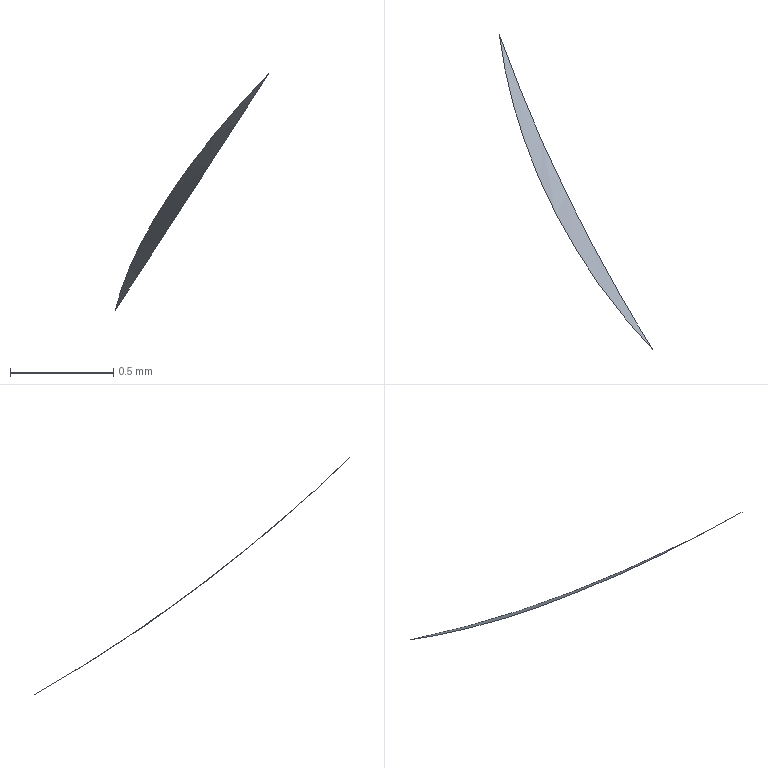Part | NX | features solid 2 | 1 solid | 2 faces | box 0.7466 x 1.533 x 1.152 mm | volume 0.001023 mm3 | cylinder 1 | spline 1 | commonest cylinder face diameters 15 x1
STEP:
#1=CARTESIAN_POINT('',(584.823,137.362,-33.981));
#2=VERTEX_POINT('',#1);
#3=CARTESIAN_POINT('',(584.077,138.895,-35.133));
#4=VERTEX_POINT('',#3);
#5=CARTESIAN_POINT('',(584.077,138.895,-35.133));
#6=CARTESIAN_POINT('',(584.194,138.576,-34.952));
#7=CARTESIAN_POINT('',(584.395,138.111,-34.642));
#8=CARTESIAN_POINT('',(584.674,137.599,-34.212));
#9=CARTESIAN_POINT('',(584.823,137.362,-33.981));
#10=B_SPLINE_CURVE_WITH_KNOTS('',3,(#5,#6,#7,#8,#9),.UNSPECIFIED.,.F.,.F.,(4,1,4),(0.4833,0.6175,0.7518),.UNSPECIFIED.);
#11=EDGE_CURVE('',#2,#4,#10,.F.);
#12=ORIENTED_EDGE('',*,*,#11,.F.);
#13=CARTESIAN_POINT('',(584.822,137.361,-33.981));
#14=CARTESIAN_POINT('',(584.437,137.772,-34.381));
#15=CARTESIAN_POINT('',(584.156,138.297,-34.794));
#16=CARTESIAN_POINT('',(584.077,138.895,-35.133));
#17=B_SPLINE_CURVE_WITH_KNOTS('',3,(#13,#14,#15,#16),.UNSPECIFIED.,.F.,.F.,(4,4),(-0.0001292,0.001944),.UNSPECIFIED.);
#18=EDGE_CURVE('',#4,#2,#17,.F.);
#19=ORIENTED_EDGE('',*,*,#18,.F.);
#20=EDGE_LOOP('',(#12,#19));
#21=FACE_BOUND('',#20,.T.);
#22=CARTESIAN_POINT('',(699.976,142.581,-28.61));
#23=DIRECTION('',(1.,-0.00013,0.000000201));
#24=DIRECTION('',(0.0001298,0.9979,0.0641));
#25=AXIS2_PLACEMENT_3D('',#22,#23,#24);
#26=CYLINDRICAL_SURFACE('',#25,7.5);
#27=ADVANCED_FACE('',(#21),#26,.T.);
#28=ORIENTED_EDGE('',*,*,#18,.T.);
#29=ORIENTED_EDGE('',*,*,#11,.T.);
#30=EDGE_LOOP('',(#28,#29));
#31=FACE_BOUND('',#30,.T.);
#32=CARTESIAN_POINT('',(584.828,137.353,-33.973));
#33=CARTESIAN_POINT('',(584.766,137.347,-33.967));
#34=CARTESIAN_POINT('',(584.704,137.341,-33.962));
#35=CARTESIAN_POINT('',(584.826,137.356,-33.976));
#36=CARTESIAN_POINT('',(584.764,137.35,-33.97));
#37=CARTESIAN_POINT('',(584.702,137.344,-33.964));
#38=CARTESIAN_POINT('',(584.824,137.359,-33.978));
#39=CARTESIAN_POINT('',(584.762,137.353,-33.973));
#40=CARTESIAN_POINT('',(584.7,137.346,-33.967));
#41=CARTESIAN_POINT('',(584.534,137.818,-34.427));
#42=CARTESIAN_POINT('',(584.472,137.813,-34.422));
#43=CARTESIAN_POINT('',(584.411,137.806,-34.417));
#44=CARTESIAN_POINT('',(584.281,138.339,-34.818));
#45=CARTESIAN_POINT('',(584.22,138.334,-34.814));
#46=CARTESIAN_POINT('',(584.158,138.328,-34.811));
#47=CARTESIAN_POINT('',(584.076,138.898,-35.135));
#48=CARTESIAN_POINT('',(584.015,138.893,-35.132));
#49=CARTESIAN_POINT('',(583.954,138.888,-35.129));
#50=CARTESIAN_POINT('',(584.074,138.901,-35.137));
#51=CARTESIAN_POINT('',(584.013,138.896,-35.134));
#52=CARTESIAN_POINT('',(583.952,138.891,-35.131));
#53=CARTESIAN_POINT('',(584.073,138.905,-35.139));
#54=CARTESIAN_POINT('',(584.012,138.899,-35.136));
#55=CARTESIAN_POINT('',(583.951,138.894,-35.133));
#56=(BOUNDED_SURFACE()B_SPLINE_SURFACE(3,2,((#32,#33,#34),(#35,#36,#37),(#38,#39,#40),(#41,#42,#43),(#44,#45,#46),(#47,#48,#49),(#50,#51,#52),(#53,#54,#55)),.UNSPECIFIED.,.F.,.F.,.F.)B_SPLINE_SURFACE_WITH_KNOTS((4,2,2,4),(3,3),(0.2485,0.25,0.5,0.5015),(0.,0.005418),.UNSPECIFIED.)GEOMETRIC_REPRESENTATION_ITEM()RATIONAL_B_SPLINE_SURFACE(((1.,0.9987,0.9973),(1.,0.9987,0.9973),(1.,0.9987,0.9973),(1.,0.9987,0.9974),(1.,0.9987,0.9974),(1.,0.9987,0.9975),(1.,0.9987,0.9975),(1.,0.9987,0.9975)))REPRESENTATION_ITEM('')SURFACE());
#57=ADVANCED_FACE('',(#31),#56,.T.);
#58=CLOSED_SHELL('',(#27,#57));
#59=MANIFOLD_SOLID_BREP('',#58);
#60=(LENGTH_UNIT()NAMED_UNIT(*)SI_UNIT(.MILLI.,.METRE.));
#61=UNCERTAINTY_MEASURE_WITH_UNIT(LENGTH_MEASURE(0.0508),#60,'','');
#62=(NAMED_UNIT(*)PLANE_ANGLE_UNIT()SI_UNIT($,.RADIAN.));
#63=(NAMED_UNIT(*)SI_UNIT($,.STERADIAN.)SOLID_ANGLE_UNIT());
#64=(GEOMETRIC_REPRESENTATION_CONTEXT(3)GLOBAL_UNCERTAINTY_ASSIGNED_CONTEXT((#61))GLOBAL_UNIT_ASSIGNED_CONTEXT((#60,#62,#63))REPRESENTATION_CONTEXT('',''));
#65=ADVANCED_BREP_SHAPE_REPRESENTATION('',(#59),#64);